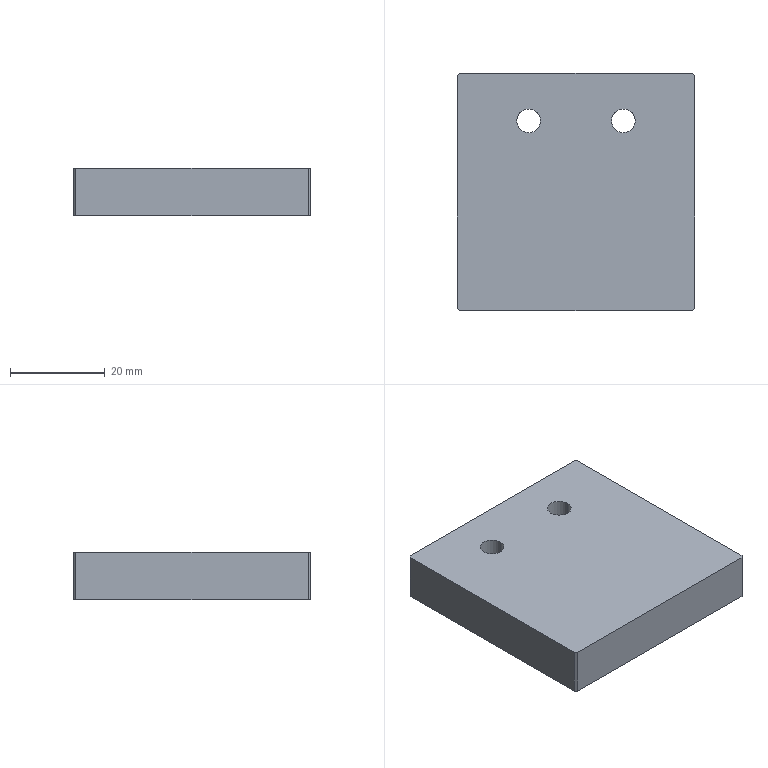Part | STEP file | 2027 Cylinder pad block | 1 solid | 14 faces | box 50 x 50 x 10 mm | volume 24602 mm3 | plane 10 | cylinder 4 | commonest cylinder face diameters 5 x4
STEP:
#1=CARTESIAN_POINT('',(0.,0.,0.));
#2=DIRECTION('',(0.,0.,1.));
#3=DIRECTION('',(1.,0.,0.));
#4=AXIS2_PLACEMENT_3D('',#1,#2,#3);
#5=CARTESIAN_POINT('',(-7.5,15.,0.));
#6=VERTEX_POINT('',#5);
#7=CARTESIAN_POINT('',(-7.5,15.,10.));
#8=VERTEX_POINT('',#7);
#9=CARTESIAN_POINT('',(-7.5,15.,10.));
#10=DIRECTION('',(0.,0.,1.));
#11=VECTOR('',#10,1.);
#12=LINE('',#9,#11);
#13=CARTESIAN_POINT('',(-10.,15.,10.));
#14=DIRECTION('',(0.,0.,1.));
#15=DIRECTION('',(1.,0.,0.));
#16=AXIS2_PLACEMENT_3D('',#13,#14,#15);
#17=CYLINDRICAL_SURFACE('',#16,2.5);
#18=CARTESIAN_POINT('',(6.283,0.));
#19=DIRECTION('',(0.,1.));
#20=VECTOR('',#19,1.);
#21=LINE('',#18,#20);
#22=(GEOMETRIC_REPRESENTATION_CONTEXT(2)PARAMETRIC_REPRESENTATION_CONTEXT()REPRESENTATION_CONTEXT('',''));
#23=DEFINITIONAL_REPRESENTATION('',(#21),#22);
#24=PCURVE('',#17,#23);
#25=CARTESIAN_POINT('',(-10.,15.,10.));
#26=DIRECTION('',(0.,0.,1.));
#27=DIRECTION('',(1.,0.,0.));
#28=AXIS2_PLACEMENT_3D('',#25,#26,#27);
#29=CYLINDRICAL_SURFACE('',#28,2.5);
#30=CARTESIAN_POINT('',(0.,0.));
#31=DIRECTION('',(0.,1.));
#32=VECTOR('',#31,1.);
#33=LINE('',#30,#32);
#34=(GEOMETRIC_REPRESENTATION_CONTEXT(2)PARAMETRIC_REPRESENTATION_CONTEXT()REPRESENTATION_CONTEXT('',''));
#35=DEFINITIONAL_REPRESENTATION('',(#33),#34);
#36=PCURVE('',#29,#35);
#37=SURFACE_CURVE('',#12,(#24,#36),.PCURVE_S1.);
#38=EDGE_CURVE('',#6,#8,#37,.T.);
#39=ORIENTED_EDGE('',*,*,#38,.T.);
#40=CARTESIAN_POINT('',(-12.5,15.,10.));
#41=VERTEX_POINT('',#40);
#42=CARTESIAN_POINT('',(-10.,15.,10.));
#43=DIRECTION('',(0.,0.,1.));
#44=DIRECTION('',(1.,0.,0.));
#45=AXIS2_PLACEMENT_3D('',#42,#43,#44);
#46=CIRCLE('',#45,2.5);
#47=CARTESIAN_POINT('',(0.,0.));
#48=DIRECTION('',(1.,0.));
#49=VECTOR('',#48,1.);
#50=LINE('',#47,#49);
#51=(GEOMETRIC_REPRESENTATION_CONTEXT(2)PARAMETRIC_REPRESENTATION_CONTEXT()REPRESENTATION_CONTEXT('',''));
#52=DEFINITIONAL_REPRESENTATION('',(#50),#51);
#53=PCURVE('',#17,#52);
#54=CARTESIAN_POINT('',(0.,0.,10.));
#55=DIRECTION('',(0.,0.,-1.));
#56=DIRECTION('',(-1.,0.,0.));
#57=AXIS2_PLACEMENT_3D('',#54,#55,#56);
#58=PLANE('',#57);
#59=CARTESIAN_POINT('',(7.5,15.));
#60=CARTESIAN_POINT('',(7.5,19.33));
#61=CARTESIAN_POINT('',(11.25,17.165));
#62=CARTESIAN_POINT('',(15.,15.));
#63=CARTESIAN_POINT('',(11.25,12.835));
#64=CARTESIAN_POINT('',(7.5,10.67));
#65=CARTESIAN_POINT('',(7.5,15.));
#66=(BOUNDED_CURVE()B_SPLINE_CURVE(2,(#59,#60,#61,#62,#63,#64,#65),.UNSPECIFIED.,.T.,.F.)B_SPLINE_CURVE_WITH_KNOTS((1,2,2,2,2,1),(-2.094,0.,2.094,4.189,6.283,8.378),.UNSPECIFIED.)CURVE()GEOMETRIC_REPRESENTATION_ITEM()RATIONAL_B_SPLINE_CURVE((1.,0.5,1.,0.5,1.,0.5,1.))REPRESENTATION_ITEM(''));
#67=(GEOMETRIC_REPRESENTATION_CONTEXT(2)PARAMETRIC_REPRESENTATION_CONTEXT()REPRESENTATION_CONTEXT('',''));
#68=DEFINITIONAL_REPRESENTATION('',(#66),#67);
#69=PCURVE('',#58,#68);
#70=SURFACE_CURVE('',#46,(#53,#69),.PCURVE_S1.);
#71=EDGE_CURVE('',#41,#8,#70,.T.);
#72=ORIENTED_EDGE('',*,*,#71,.F.);
#73=CARTESIAN_POINT('',(-12.5,15.,0.));
#74=VERTEX_POINT('',#73);
#75=CARTESIAN_POINT('',(-12.5,15.,10.));
#76=DIRECTION('',(0.,0.,1.));
#77=VECTOR('',#76,1.);
#78=LINE('',#75,#77);
#79=CARTESIAN_POINT('',(3.142,0.));
#80=DIRECTION('',(0.,1.));
#81=VECTOR('',#80,1.);
#82=LINE('',#79,#81);
#83=(GEOMETRIC_REPRESENTATION_CONTEXT(2)PARAMETRIC_REPRESENTATION_CONTEXT()REPRESENTATION_CONTEXT('',''));
#84=DEFINITIONAL_REPRESENTATION('',(#82),#83);
#85=PCURVE('',#17,#84);
#86=CARTESIAN_POINT('',(3.142,0.));
#87=DIRECTION('',(0.,1.));
#88=VECTOR('',#87,1.);
#89=LINE('',#86,#88);
#90=(GEOMETRIC_REPRESENTATION_CONTEXT(2)PARAMETRIC_REPRESENTATION_CONTEXT()REPRESENTATION_CONTEXT('',''));
#91=DEFINITIONAL_REPRESENTATION('',(#89),#90);
#92=PCURVE('',#29,#91);
#93=SURFACE_CURVE('',#78,(#85,#92),.PCURVE_S1.);
#94=EDGE_CURVE('',#74,#41,#93,.T.);
#95=ORIENTED_EDGE('',*,*,#94,.F.);
#96=CARTESIAN_POINT('',(-10.,15.,0.));
#97=DIRECTION('',(0.,0.,1.));
#98=DIRECTION('',(1.,0.,0.));
#99=AXIS2_PLACEMENT_3D('',#96,#97,#98);
#100=CIRCLE('',#99,2.5);
#101=CARTESIAN_POINT('',(0.,-10.));
#102=DIRECTION('',(1.,0.));
#103=VECTOR('',#102,1.);
#104=LINE('',#101,#103);
#105=(GEOMETRIC_REPRESENTATION_CONTEXT(2)PARAMETRIC_REPRESENTATION_CONTEXT()REPRESENTATION_CONTEXT('',''));
#106=DEFINITIONAL_REPRESENTATION('',(#104),#105);
#107=PCURVE('',#17,#106);
#108=CARTESIAN_POINT('',(0.,0.,0.));
#109=DIRECTION('',(0.,0.,-1.));
#110=DIRECTION('',(-1.,0.,0.));
#111=AXIS2_PLACEMENT_3D('',#108,#109,#110);
#112=PLANE('',#111);
#113=CARTESIAN_POINT('',(7.5,15.));
#114=CARTESIAN_POINT('',(7.5,19.33));
#115=CARTESIAN_POINT('',(11.25,17.165));
#116=CARTESIAN_POINT('',(15.,15.));
#117=CARTESIAN_POINT('',(11.25,12.835));
#118=CARTESIAN_POINT('',(7.5,10.67));
#119=CARTESIAN_POINT('',(7.5,15.));
#120=(BOUNDED_CURVE()B_SPLINE_CURVE(2,(#113,#114,#115,#116,#117,#118,#119),.UNSPECIFIED.,.T.,.F.)B_SPLINE_CURVE_WITH_KNOTS((1,2,2,2,2,1),(-2.094,0.,2.094,4.189,6.283,8.378),.UNSPECIFIED.)CURVE()GEOMETRIC_REPRESENTATION_ITEM()RATIONAL_B_SPLINE_CURVE((1.,0.5,1.,0.5,1.,0.5,1.))REPRESENTATION_ITEM(''));
#121=(GEOMETRIC_REPRESENTATION_CONTEXT(2)PARAMETRIC_REPRESENTATION_CONTEXT()REPRESENTATION_CONTEXT('',''));
#122=DEFINITIONAL_REPRESENTATION('',(#120),#121);
#123=PCURVE('',#112,#122);
#124=SURFACE_CURVE('',#100,(#107,#123),.PCURVE_S1.);
#125=EDGE_CURVE('',#74,#6,#124,.T.);
#126=ORIENTED_EDGE('',*,*,#125,.T.);
#127=EDGE_LOOP('',(#39,#72,#95,#126));
#128=FACE_BOUND('',#127,.F.);
#129=ADVANCED_FACE('',(#128),#17,.F.);
#130=CARTESIAN_POINT('',(12.5,15.,0.));
#131=VERTEX_POINT('',#130);
#132=CARTESIAN_POINT('',(12.5,15.,10.));
#133=VERTEX_POINT('',#132);
#134=CARTESIAN_POINT('',(12.5,15.,10.));
#135=DIRECTION('',(0.,0.,1.));
#136=VECTOR('',#135,1.);
#137=LINE('',#134,#136);
#138=CARTESIAN_POINT('',(10.,15.,10.));
#139=DIRECTION('',(0.,0.,1.));
#140=DIRECTION('',(1.,0.,0.));
#141=AXIS2_PLACEMENT_3D('',#138,#139,#140);
#142=CYLINDRICAL_SURFACE('',#141,2.5);
#143=CARTESIAN_POINT('',(6.283,0.));
#144=DIRECTION('',(0.,1.));
#145=VECTOR('',#144,1.);
#146=LINE('',#143,#145);
#147=(GEOMETRIC_REPRESENTATION_CONTEXT(2)PARAMETRIC_REPRESENTATION_CONTEXT()REPRESENTATION_CONTEXT('',''));
#148=DEFINITIONAL_REPRESENTATION('',(#146),#147);
#149=PCURVE('',#142,#148);
#150=CARTESIAN_POINT('',(10.,15.,10.));
#151=DIRECTION('',(0.,0.,1.));
#152=DIRECTION('',(1.,0.,0.));
#153=AXIS2_PLACEMENT_3D('',#150,#151,#152);
#154=CYLINDRICAL_SURFACE('',#153,2.5);
#155=CARTESIAN_POINT('',(0.,0.));
#156=DIRECTION('',(0.,1.));
#157=VECTOR('',#156,1.);
#158=LINE('',#155,#157);
#159=(GEOMETRIC_REPRESENTATION_CONTEXT(2)PARAMETRIC_REPRESENTATION_CONTEXT()REPRESENTATION_CONTEXT('',''));
#160=DEFINITIONAL_REPRESENTATION('',(#158),#159);
#161=PCURVE('',#154,#160);
#162=SURFACE_CURVE('',#137,(#149,#161),.PCURVE_S1.);
#163=EDGE_CURVE('',#131,#133,#162,.T.);
#164=ORIENTED_EDGE('',*,*,#163,.T.);
#165=CARTESIAN_POINT('',(7.5,15.,10.));
#166=VERTEX_POINT('',#165);
#167=CARTESIAN_POINT('',(10.,15.,10.));
#168=DIRECTION('',(0.,0.,1.));
#169=DIRECTION('',(1.,0.,0.));
#170=AXIS2_PLACEMENT_3D('',#167,#168,#169);
#171=CIRCLE('',#170,2.5);
#172=CARTESIAN_POINT('',(0.,0.));
#173=DIRECTION('',(1.,0.));
#174=VECTOR('',#173,1.);
#175=LINE('',#172,#174);
#176=(GEOMETRIC_REPRESENTATION_CONTEXT(2)PARAMETRIC_REPRESENTATION_CONTEXT()REPRESENTATION_CONTEXT('',''));
#177=DEFINITIONAL_REPRESENTATION('',(#175),#176);
#178=PCURVE('',#142,#177);
#179=CARTESIAN_POINT('',(-12.5,15.));
#180=CARTESIAN_POINT('',(-12.5,19.33));
#181=CARTESIAN_POINT('',(-8.75,17.165));
#182=CARTESIAN_POINT('',(-5.,15.));
#183=CARTESIAN_POINT('',(-8.75,12.835));
#184=CARTESIAN_POINT('',(-12.5,10.67));
#185=CARTESIAN_POINT('',(-12.5,15.));
#186=(BOUNDED_CURVE()B_SPLINE_CURVE(2,(#179,#180,#181,#182,#183,#184,#185),.UNSPECIFIED.,.T.,.F.)B_SPLINE_CURVE_WITH_KNOTS((1,2,2,2,2,1),(-2.094,0.,2.094,4.189,6.283,8.378),.UNSPECIFIED.)CURVE()GEOMETRIC_REPRESENTATION_ITEM()RATIONAL_B_SPLINE_CURVE((1.,0.5,1.,0.5,1.,0.5,1.))REPRESENTATION_ITEM(''));
#187=(GEOMETRIC_REPRESENTATION_CONTEXT(2)PARAMETRIC_REPRESENTATION_CONTEXT()REPRESENTATION_CONTEXT('',''));
#188=DEFINITIONAL_REPRESENTATION('',(#186),#187);
#189=PCURVE('',#58,#188);
#190=SURFACE_CURVE('',#171,(#178,#189),.PCURVE_S1.);
#191=EDGE_CURVE('',#166,#133,#190,.T.);
#192=ORIENTED_EDGE('',*,*,#191,.F.);
#193=CARTESIAN_POINT('',(7.5,15.,0.));
#194=VERTEX_POINT('',#193);
#195=CARTESIAN_POINT('',(7.5,15.,10.));
#196=DIRECTION('',(0.,0.,1.));
#197=VECTOR('',#196,1.);
#198=LINE('',#195,#197);
#199=CARTESIAN_POINT('',(3.142,0.));
#200=DIRECTION('',(0.,1.));
#201=VECTOR('',#200,1.);
#202=LINE('',#199,#201);
#203=(GEOMETRIC_REPRESENTATION_CONTEXT(2)PARAMETRIC_REPRESENTATION_CONTEXT()REPRESENTATION_CONTEXT('',''));
#204=DEFINITIONAL_REPRESENTATION('',(#202),#203);
#205=PCURVE('',#142,#204);
#206=CARTESIAN_POINT('',(3.142,0.));
#207=DIRECTION('',(0.,1.));
#208=VECTOR('',#207,1.);
#209=LINE('',#206,#208);
#210=(GEOMETRIC_REPRESENTATION_CONTEXT(2)PARAMETRIC_REPRESENTATION_CONTEXT()REPRESENTATION_CONTEXT('',''));
#211=DEFINITIONAL_REPRESENTATION('',(#209),#210);
#212=PCURVE('',#154,#211);
#213=SURFACE_CURVE('',#198,(#205,#212),.PCURVE_S1.);
#214=EDGE_CURVE('',#194,#166,#213,.T.);
#215=ORIENTED_EDGE('',*,*,#214,.F.);
#216=CARTESIAN_POINT('',(10.,15.,0.));
#217=DIRECTION('',(0.,0.,1.));
#218=DIRECTION('',(1.,0.,0.));
#219=AXIS2_PLACEMENT_3D('',#216,#217,#218);
#220=CIRCLE('',#219,2.5);
#221=CARTESIAN_POINT('',(0.,-10.));
#222=DIRECTION('',(1.,0.));
#223=VECTOR('',#222,1.);
#224=LINE('',#221,#223);
#225=(GEOMETRIC_REPRESENTATION_CONTEXT(2)PARAMETRIC_REPRESENTATION_CONTEXT()REPRESENTATION_CONTEXT('',''));
#226=DEFINITIONAL_REPRESENTATION('',(#224),#225);
#227=PCURVE('',#142,#226);
#228=CARTESIAN_POINT('',(-12.5,15.));
#229=CARTESIAN_POINT('',(-12.5,19.33));
#230=CARTESIAN_POINT('',(-8.75,17.165));
#231=CARTESIAN_POINT('',(-5.,15.));
#232=CARTESIAN_POINT('',(-8.75,12.835));
#233=CARTESIAN_POINT('',(-12.5,10.67));
#234=CARTESIAN_POINT('',(-12.5,15.));
#235=(BOUNDED_CURVE()B_SPLINE_CURVE(2,(#228,#229,#230,#231,#232,#233,#234),.UNSPECIFIED.,.T.,.F.)B_SPLINE_CURVE_WITH_KNOTS((1,2,2,2,2,1),(-2.094,0.,2.094,4.189,6.283,8.378),.UNSPECIFIED.)CURVE()GEOMETRIC_REPRESENTATION_ITEM()RATIONAL_B_SPLINE_CURVE((1.,0.5,1.,0.5,1.,0.5,1.))REPRESENTATION_ITEM(''));
#236=(GEOMETRIC_REPRESENTATION_CONTEXT(2)PARAMETRIC_REPRESENTATION_CONTEXT()REPRESENTATION_CONTEXT('',''));
#237=DEFINITIONAL_REPRESENTATION('',(#235),#236);
#238=PCURVE('',#112,#237);
#239=SURFACE_CURVE('',#220,(#227,#238),.PCURVE_S1.);
#240=EDGE_CURVE('',#194,#131,#239,.T.);
#241=ORIENTED_EDGE('',*,*,#240,.T.);
#242=EDGE_LOOP('',(#164,#192,#215,#241));
#243=FACE_BOUND('',#242,.F.);
#244=ADVANCED_FACE('',(#243),#142,.F.);
#245=CARTESIAN_POINT('',(25.,-24.5,0.));
#246=VERTEX_POINT('',#245);
#247=CARTESIAN_POINT('',(25.,24.5,0.));
#248=VERTEX_POINT('',#247);
#249=CARTESIAN_POINT('',(25.,-25.,0.));
#250=DIRECTION('',(0.,1.,0.));
#251=VECTOR('',#250,1.);
#252=LINE('',#249,#251);
#253=CARTESIAN_POINT('',(25.,-25.,10.));
#254=DIRECTION('',(-1.,0.,0.));
#255=DIRECTION('',(0.,0.,1.));
#256=AXIS2_PLACEMENT_3D('',#253,#254,#255);
#257=PLANE('',#256);
#258=CARTESIAN_POINT('',(-10.,0.));
#259=DIRECTION('',(0.,1.));
#260=VECTOR('',#259,1.);
#261=LINE('',#258,#260);
#262=(GEOMETRIC_REPRESENTATION_CONTEXT(2)PARAMETRIC_REPRESENTATION_CONTEXT()REPRESENTATION_CONTEXT('',''));
#263=DEFINITIONAL_REPRESENTATION('',(#261),#262);
#264=PCURVE('',#257,#263);
#265=CARTESIAN_POINT('',(-25.,-25.));
#266=DIRECTION('',(0.,1.));
#267=VECTOR('',#266,1.);
#268=LINE('',#265,#267);
#269=(GEOMETRIC_REPRESENTATION_CONTEXT(2)PARAMETRIC_REPRESENTATION_CONTEXT()REPRESENTATION_CONTEXT('',''));
#270=DEFINITIONAL_REPRESENTATION('',(#268),#269);
#271=PCURVE('',#112,#270);
#272=SURFACE_CURVE('',#252,(#264,#271),.PCURVE_S1.);
#273=EDGE_CURVE('',#246,#248,#272,.T.);
#274=ORIENTED_EDGE('',*,*,#273,.T.);
#275=CARTESIAN_POINT('',(25.,24.5,10.));
#276=VERTEX_POINT('',#275);
#277=CARTESIAN_POINT('',(25.,24.5,10.));
#278=DIRECTION('',(0.,0.,1.));
#279=VECTOR('',#278,1.);
#280=LINE('',#277,#279);
#281=CARTESIAN_POINT('',(0.,49.5));
#282=DIRECTION('',(1.,0.));
#283=VECTOR('',#282,1.);
#284=LINE('',#281,#283);
#285=(GEOMETRIC_REPRESENTATION_CONTEXT(2)PARAMETRIC_REPRESENTATION_CONTEXT()REPRESENTATION_CONTEXT('',''));
#286=DEFINITIONAL_REPRESENTATION('',(#284),#285);
#287=PCURVE('',#257,#286);
#288=CARTESIAN_POINT('',(24.5,25.,10.));
#289=DIRECTION('',(-0.7071,-0.7071,0.));
#290=DIRECTION('',(0.,0.,-1.));
#291=AXIS2_PLACEMENT_3D('',#288,#289,#290);
#292=PLANE('',#291);
#293=CARTESIAN_POINT('',(0.,0.7071));
#294=DIRECTION('',(-1.,0.));
#295=VECTOR('',#294,1.);
#296=LINE('',#293,#295);
#297=(GEOMETRIC_REPRESENTATION_CONTEXT(2)PARAMETRIC_REPRESENTATION_CONTEXT()REPRESENTATION_CONTEXT('',''));
#298=DEFINITIONAL_REPRESENTATION('',(#296),#297);
#299=PCURVE('',#292,#298);
#300=SURFACE_CURVE('',#280,(#287,#299),.PCURVE_S1.);
#301=EDGE_CURVE('',#248,#276,#300,.T.);
#302=ORIENTED_EDGE('',*,*,#301,.T.);
#303=CARTESIAN_POINT('',(25.,-24.5,10.));
#304=VERTEX_POINT('',#303);
#305=CARTESIAN_POINT('',(25.,-25.,10.));
#306=DIRECTION('',(0.,1.,0.));
#307=VECTOR('',#306,1.);
#308=LINE('',#305,#307);
#309=CARTESIAN_POINT('',(0.,0.));
#310=DIRECTION('',(0.,1.));
#311=VECTOR('',#310,1.);
#312=LINE('',#309,#311);
#313=(GEOMETRIC_REPRESENTATION_CONTEXT(2)PARAMETRIC_REPRESENTATION_CONTEXT()REPRESENTATION_CONTEXT('',''));
#314=DEFINITIONAL_REPRESENTATION('',(#312),#313);
#315=PCURVE('',#257,#314);
#316=CARTESIAN_POINT('',(-25.,-25.));
#317=DIRECTION('',(0.,1.));
#318=VECTOR('',#317,1.);
#319=LINE('',#316,#318);
#320=(GEOMETRIC_REPRESENTATION_CONTEXT(2)PARAMETRIC_REPRESENTATION_CONTEXT()REPRESENTATION_CONTEXT('',''));
#321=DEFINITIONAL_REPRESENTATION('',(#319),#320);
#322=PCURVE('',#58,#321);
#323=SURFACE_CURVE('',#308,(#315,#322),.PCURVE_S1.);
#324=EDGE_CURVE('',#304,#276,#323,.T.);
#325=ORIENTED_EDGE('',*,*,#324,.F.);
#326=CARTESIAN_POINT('',(25.,-24.5,10.));
#327=DIRECTION('',(0.,0.,-1.));
#328=VECTOR('',#327,1.);
#329=LINE('',#326,#328);
#330=CARTESIAN_POINT('',(0.,0.5));
#331=DIRECTION('',(-1.,0.));
#332=VECTOR('',#331,1.);
#333=LINE('',#330,#332);
#334=(GEOMETRIC_REPRESENTATION_CONTEXT(2)PARAMETRIC_REPRESENTATION_CONTEXT()REPRESENTATION_CONTEXT('',''));
#335=DEFINITIONAL_REPRESENTATION('',(#333),#334);
#336=PCURVE('',#257,#335);
#337=CARTESIAN_POINT('',(25.,-24.5,10.));
#338=DIRECTION('',(-0.7071,0.7071,0.));
#339=DIRECTION('',(0.,0.,-1.));
#340=AXIS2_PLACEMENT_3D('',#337,#338,#339);
#341=PLANE('',#340);
#342=CARTESIAN_POINT('',(0.,0.));
#343=DIRECTION('',(1.,0.));
#344=VECTOR('',#343,1.);
#345=LINE('',#342,#344);
#346=(GEOMETRIC_REPRESENTATION_CONTEXT(2)PARAMETRIC_REPRESENTATION_CONTEXT()REPRESENTATION_CONTEXT('',''));
#347=DEFINITIONAL_REPRESENTATION('',(#345),#346);
#348=PCURVE('',#341,#347);
#349=SURFACE_CURVE('',#329,(#336,#348),.PCURVE_S1.);
#350=EDGE_CURVE('',#304,#246,#349,.T.);
#351=ORIENTED_EDGE('',*,*,#350,.T.);
#352=EDGE_LOOP('',(#274,#302,#325,#351));
#353=FACE_BOUND('',#352,.T.);
#354=ADVANCED_FACE('',(#353),#257,.F.);
#355=CARTESIAN_POINT('',(24.5,25.,10.));
#356=VERTEX_POINT('',#355);
#357=CARTESIAN_POINT('',(-24.5,25.,10.));
#358=VERTEX_POINT('',#357);
#359=CARTESIAN_POINT('',(-25.,25.,10.));
#360=DIRECTION('',(-1.,0.,0.));
#361=VECTOR('',#360,1.);
#362=LINE('',#359,#361);
#363=CARTESIAN_POINT('',(-25.,25.,10.));
#364=DIRECTION('',(0.,-1.,0.));
#365=DIRECTION('',(0.,0.,-1.));
#366=AXIS2_PLACEMENT_3D('',#363,#364,#365);
#367=PLANE('',#366);
#368=CARTESIAN_POINT('',(0.,0.));
#369=DIRECTION('',(0.,-1.));
#370=VECTOR('',#369,1.);
#371=LINE('',#368,#370);
#372=(GEOMETRIC_REPRESENTATION_CONTEXT(2)PARAMETRIC_REPRESENTATION_CONTEXT()REPRESENTATION_CONTEXT('',''));
#373=DEFINITIONAL_REPRESENTATION('',(#371),#372);
#374=PCURVE('',#367,#373);
#375=CARTESIAN_POINT('',(25.,25.));
#376=DIRECTION('',(1.,0.));
#377=VECTOR('',#376,1.);
#378=LINE('',#375,#377);
#379=(GEOMETRIC_REPRESENTATION_CONTEXT(2)PARAMETRIC_REPRESENTATION_CONTEXT()REPRESENTATION_CONTEXT('',''));
#380=DEFINITIONAL_REPRESENTATION('',(#378),#379);
#381=PCURVE('',#58,#380);
#382=SURFACE_CURVE('',#362,(#374,#381),.PCURVE_S1.);
#383=EDGE_CURVE('',#356,#358,#382,.T.);
#384=ORIENTED_EDGE('',*,*,#383,.F.);
#385=CARTESIAN_POINT('',(24.5,25.,0.));
#386=VERTEX_POINT('',#385);
#387=CARTESIAN_POINT('',(24.5,25.,10.));
#388=DIRECTION('',(0.,0.,-1.));
#389=VECTOR('',#388,1.);
#390=LINE('',#387,#389);
#391=CARTESIAN_POINT('',(0.,49.5));
#392=DIRECTION('',(1.,0.));
#393=VECTOR('',#392,1.);
#394=LINE('',#391,#393);
#395=(GEOMETRIC_REPRESENTATION_CONTEXT(2)PARAMETRIC_REPRESENTATION_CONTEXT()REPRESENTATION_CONTEXT('',''));
#396=DEFINITIONAL_REPRESENTATION('',(#394),#395);
#397=PCURVE('',#367,#396);
#398=CARTESIAN_POINT('',(0.,0.));
#399=DIRECTION('',(1.,0.));
#400=VECTOR('',#399,1.);
#401=LINE('',#398,#400);
#402=(GEOMETRIC_REPRESENTATION_CONTEXT(2)PARAMETRIC_REPRESENTATION_CONTEXT()REPRESENTATION_CONTEXT('',''));
#403=DEFINITIONAL_REPRESENTATION('',(#401),#402);
#404=PCURVE('',#292,#403);
#405=SURFACE_CURVE('',#390,(#397,#404),.PCURVE_S1.);
#406=EDGE_CURVE('',#356,#386,#405,.T.);
#407=ORIENTED_EDGE('',*,*,#406,.T.);
#408=CARTESIAN_POINT('',(-24.5,25.,0.));
#409=VERTEX_POINT('',#408);
#410=CARTESIAN_POINT('',(-25.,25.,0.));
#411=DIRECTION('',(-1.,0.,0.));
#412=VECTOR('',#411,1.);
#413=LINE('',#410,#412);
#414=CARTESIAN_POINT('',(10.,0.));
#415=DIRECTION('',(0.,-1.));
#416=VECTOR('',#415,1.);
#417=LINE('',#414,#416);
#418=(GEOMETRIC_REPRESENTATION_CONTEXT(2)PARAMETRIC_REPRESENTATION_CONTEXT()REPRESENTATION_CONTEXT('',''));
#419=DEFINITIONAL_REPRESENTATION('',(#417),#418);
#420=PCURVE('',#367,#419);
#421=CARTESIAN_POINT('',(25.,25.));
#422=DIRECTION('',(1.,0.));
#423=VECTOR('',#422,1.);
#424=LINE('',#421,#423);
#425=(GEOMETRIC_REPRESENTATION_CONTEXT(2)PARAMETRIC_REPRESENTATION_CONTEXT()REPRESENTATION_CONTEXT('',''));
#426=DEFINITIONAL_REPRESENTATION('',(#424),#425);
#427=PCURVE('',#112,#426);
#428=SURFACE_CURVE('',#413,(#420,#427),.PCURVE_S1.);
#429=EDGE_CURVE('',#386,#409,#428,.T.);
#430=ORIENTED_EDGE('',*,*,#429,.T.);
#431=CARTESIAN_POINT('',(-24.5,25.,10.));
#432=DIRECTION('',(0.,0.,1.));
#433=VECTOR('',#432,1.);
#434=LINE('',#431,#433);
#435=CARTESIAN_POINT('',(0.,0.5));
#436=DIRECTION('',(-1.,0.));
#437=VECTOR('',#436,1.);
#438=LINE('',#435,#437);
#439=(GEOMETRIC_REPRESENTATION_CONTEXT(2)PARAMETRIC_REPRESENTATION_CONTEXT()REPRESENTATION_CONTEXT('',''));
#440=DEFINITIONAL_REPRESENTATION('',(#438),#439);
#441=PCURVE('',#367,#440);
#442=CARTESIAN_POINT('',(-25.,24.5,10.));
#443=DIRECTION('',(0.7071,-0.7071,0.));
#444=DIRECTION('',(0.,0.,-1.));
#445=AXIS2_PLACEMENT_3D('',#442,#443,#444);
#446=PLANE('',#445);
#447=CARTESIAN_POINT('',(0.,0.7071));
#448=DIRECTION('',(-1.,0.));
#449=VECTOR('',#448,1.);
#450=LINE('',#447,#449);
#451=(GEOMETRIC_REPRESENTATION_CONTEXT(2)PARAMETRIC_REPRESENTATION_CONTEXT()REPRESENTATION_CONTEXT('',''));
#452=DEFINITIONAL_REPRESENTATION('',(#450),#451);
#453=PCURVE('',#446,#452);
#454=SURFACE_CURVE('',#434,(#441,#453),.PCURVE_S1.);
#455=EDGE_CURVE('',#409,#358,#454,.T.);
#456=ORIENTED_EDGE('',*,*,#455,.T.);
#457=EDGE_LOOP('',(#384,#407,#430,#456));
#458=FACE_BOUND('',#457,.T.);
#459=ADVANCED_FACE('',(#458),#367,.F.);
#460=CARTESIAN_POINT('',(-25.,24.5,0.));
#461=VERTEX_POINT('',#460);
#462=CARTESIAN_POINT('',(-25.,-24.5,0.));
#463=VERTEX_POINT('',#462);
#464=CARTESIAN_POINT('',(-25.,-25.,0.));
#465=DIRECTION('',(0.,-1.,0.));
#466=VECTOR('',#465,1.);
#467=LINE('',#464,#466);
#468=CARTESIAN_POINT('',(-25.,-25.,10.));
#469=DIRECTION('',(1.,0.,0.));
#470=DIRECTION('',(0.,0.,-1.));
#471=AXIS2_PLACEMENT_3D('',#468,#469,#470);
#472=PLANE('',#471);
#473=CARTESIAN_POINT('',(10.,0.));
#474=DIRECTION('',(0.,-1.));
#475=VECTOR('',#474,1.);
#476=LINE('',#473,#475);
#477=(GEOMETRIC_REPRESENTATION_CONTEXT(2)PARAMETRIC_REPRESENTATION_CONTEXT()REPRESENTATION_CONTEXT('',''));
#478=DEFINITIONAL_REPRESENTATION('',(#476),#477);
#479=PCURVE('',#472,#478);
#480=CARTESIAN_POINT('',(25.,-25.));
#481=DIRECTION('',(0.,-1.));
#482=VECTOR('',#481,1.);
#483=LINE('',#480,#482);
#484=(GEOMETRIC_REPRESENTATION_CONTEXT(2)PARAMETRIC_REPRESENTATION_CONTEXT()REPRESENTATION_CONTEXT('',''));
#485=DEFINITIONAL_REPRESENTATION('',(#483),#484);
#486=PCURVE('',#112,#485);
#487=SURFACE_CURVE('',#467,(#479,#486),.PCURVE_S1.);
#488=EDGE_CURVE('',#461,#463,#487,.T.);
#489=ORIENTED_EDGE('',*,*,#488,.T.);
#490=CARTESIAN_POINT('',(-25.,-24.5,10.));
#491=VERTEX_POINT('',#490);
#492=CARTESIAN_POINT('',(-25.,-24.5,10.));
#493=DIRECTION('',(0.,0.,1.));
#494=VECTOR('',#493,1.);
#495=LINE('',#492,#494);
#496=CARTESIAN_POINT('',(0.,0.5));
#497=DIRECTION('',(-1.,0.));
#498=VECTOR('',#497,1.);
#499=LINE('',#496,#498);
#500=(GEOMETRIC_REPRESENTATION_CONTEXT(2)PARAMETRIC_REPRESENTATION_CONTEXT()REPRESENTATION_CONTEXT('',''));
#501=DEFINITIONAL_REPRESENTATION('',(#499),#500);
#502=PCURVE('',#472,#501);
#503=CARTESIAN_POINT('',(-24.5,-25.,10.));
#504=DIRECTION('',(0.7071,0.7071,0.));
#505=DIRECTION('',(0.,0.,-1.));
#506=AXIS2_PLACEMENT_3D('',#503,#504,#505);
#507=PLANE('',#506);
#508=CARTESIAN_POINT('',(0.,0.7071));
#509=DIRECTION('',(-1.,0.));
#510=VECTOR('',#509,1.);
#511=LINE('',#508,#510);
#512=(GEOMETRIC_REPRESENTATION_CONTEXT(2)PARAMETRIC_REPRESENTATION_CONTEXT()REPRESENTATION_CONTEXT('',''));
#513=DEFINITIONAL_REPRESENTATION('',(#511),#512);
#514=PCURVE('',#507,#513);
#515=SURFACE_CURVE('',#495,(#502,#514),.PCURVE_S1.);
#516=EDGE_CURVE('',#463,#491,#515,.T.);
#517=ORIENTED_EDGE('',*,*,#516,.T.);
#518=CARTESIAN_POINT('',(-25.,24.5,10.));
#519=VERTEX_POINT('',#518);
#520=CARTESIAN_POINT('',(-25.,-25.,10.));
#521=DIRECTION('',(0.,-1.,0.));
#522=VECTOR('',#521,1.);
#523=LINE('',#520,#522);
#524=CARTESIAN_POINT('',(0.,0.));
#525=DIRECTION('',(0.,-1.));
#526=VECTOR('',#525,1.);
#527=LINE('',#524,#526);
#528=(GEOMETRIC_REPRESENTATION_CONTEXT(2)PARAMETRIC_REPRESENTATION_CONTEXT()REPRESENTATION_CONTEXT('',''));
#529=DEFINITIONAL_REPRESENTATION('',(#527),#528);
#530=PCURVE('',#472,#529);
#531=CARTESIAN_POINT('',(25.,-25.));
#532=DIRECTION('',(0.,-1.));
#533=VECTOR('',#532,1.);
#534=LINE('',#531,#533);
#535=(GEOMETRIC_REPRESENTATION_CONTEXT(2)PARAMETRIC_REPRESENTATION_CONTEXT()REPRESENTATION_CONTEXT('',''));
#536=DEFINITIONAL_REPRESENTATION('',(#534),#535);
#537=PCURVE('',#58,#536);
#538=SURFACE_CURVE('',#523,(#530,#537),.PCURVE_S1.);
#539=EDGE_CURVE('',#519,#491,#538,.T.);
#540=ORIENTED_EDGE('',*,*,#539,.F.);
#541=CARTESIAN_POINT('',(-25.,24.5,10.));
#542=DIRECTION('',(0.,0.,-1.));
#543=VECTOR('',#542,1.);
#544=LINE('',#541,#543);
#545=CARTESIAN_POINT('',(0.,49.5));
#546=DIRECTION('',(1.,0.));
#547=VECTOR('',#546,1.);
#548=LINE('',#545,#547);
#549=(GEOMETRIC_REPRESENTATION_CONTEXT(2)PARAMETRIC_REPRESENTATION_CONTEXT()REPRESENTATION_CONTEXT('',''));
#550=DEFINITIONAL_REPRESENTATION('',(#548),#549);
#551=PCURVE('',#472,#550);
#552=CARTESIAN_POINT('',(0.,0.));
#553=DIRECTION('',(1.,0.));
#554=VECTOR('',#553,1.);
#555=LINE('',#552,#554);
#556=(GEOMETRIC_REPRESENTATION_CONTEXT(2)PARAMETRIC_REPRESENTATION_CONTEXT()REPRESENTATION_CONTEXT('',''));
#557=DEFINITIONAL_REPRESENTATION('',(#555),#556);
#558=PCURVE('',#446,#557);
#559=SURFACE_CURVE('',#544,(#551,#558),.PCURVE_S1.);
#560=EDGE_CURVE('',#519,#461,#559,.T.);
#561=ORIENTED_EDGE('',*,*,#560,.T.);
#562=EDGE_LOOP('',(#489,#517,#540,#561));
#563=FACE_BOUND('',#562,.T.);
#564=ADVANCED_FACE('',(#563),#472,.F.);
#565=CARTESIAN_POINT('',(-24.5,-25.,0.));
#566=VERTEX_POINT('',#565);
#567=CARTESIAN_POINT('',(24.5,-25.,0.));
#568=VERTEX_POINT('',#567);
#569=CARTESIAN_POINT('',(-25.,-25.,0.));
#570=DIRECTION('',(1.,0.,0.));
#571=VECTOR('',#570,1.);
#572=LINE('',#569,#571);
#573=CARTESIAN_POINT('',(-25.,-25.,10.));
#574=DIRECTION('',(0.,1.,0.));
#575=DIRECTION('',(0.,0.,1.));
#576=AXIS2_PLACEMENT_3D('',#573,#574,#575);
#577=PLANE('',#576);
#578=CARTESIAN_POINT('',(-10.,0.));
#579=DIRECTION('',(0.,1.));
#580=VECTOR('',#579,1.);
#581=LINE('',#578,#580);
#582=(GEOMETRIC_REPRESENTATION_CONTEXT(2)PARAMETRIC_REPRESENTATION_CONTEXT()REPRESENTATION_CONTEXT('',''));
#583=DEFINITIONAL_REPRESENTATION('',(#581),#582);
#584=PCURVE('',#577,#583);
#585=CARTESIAN_POINT('',(25.,-25.));
#586=DIRECTION('',(-1.,0.));
#587=VECTOR('',#586,1.);
#588=LINE('',#585,#587);
#589=(GEOMETRIC_REPRESENTATION_CONTEXT(2)PARAMETRIC_REPRESENTATION_CONTEXT()REPRESENTATION_CONTEXT('',''));
#590=DEFINITIONAL_REPRESENTATION('',(#588),#589);
#591=PCURVE('',#112,#590);
#592=SURFACE_CURVE('',#572,(#584,#591),.PCURVE_S1.);
#593=EDGE_CURVE('',#566,#568,#592,.T.);
#594=ORIENTED_EDGE('',*,*,#593,.T.);
#595=CARTESIAN_POINT('',(24.5,-25.,10.));
#596=VERTEX_POINT('',#595);
#597=CARTESIAN_POINT('',(24.5,-25.,10.));
#598=DIRECTION('',(0.,0.,1.));
#599=VECTOR('',#598,1.);
#600=LINE('',#597,#599);
#601=CARTESIAN_POINT('',(0.,49.5));
#602=DIRECTION('',(1.,0.));
#603=VECTOR('',#602,1.);
#604=LINE('',#601,#603);
#605=(GEOMETRIC_REPRESENTATION_CONTEXT(2)PARAMETRIC_REPRESENTATION_CONTEXT()REPRESENTATION_CONTEXT('',''));
#606=DEFINITIONAL_REPRESENTATION('',(#604),#605);
#607=PCURVE('',#577,#606);
#608=CARTESIAN_POINT('',(0.,0.7071));
#609=DIRECTION('',(-1.,0.));
#610=VECTOR('',#609,1.);
#611=LINE('',#608,#610);
#612=(GEOMETRIC_REPRESENTATION_CONTEXT(2)PARAMETRIC_REPRESENTATION_CONTEXT()REPRESENTATION_CONTEXT('',''));
#613=DEFINITIONAL_REPRESENTATION('',(#611),#612);
#614=PCURVE('',#341,#613);
#615=SURFACE_CURVE('',#600,(#607,#614),.PCURVE_S1.);
#616=EDGE_CURVE('',#568,#596,#615,.T.);
#617=ORIENTED_EDGE('',*,*,#616,.T.);
#618=CARTESIAN_POINT('',(-24.5,-25.,10.));
#619=VERTEX_POINT('',#618);
#620=CARTESIAN_POINT('',(-25.,-25.,10.));
#621=DIRECTION('',(1.,0.,0.));
#622=VECTOR('',#621,1.);
#623=LINE('',#620,#622);
#624=CARTESIAN_POINT('',(0.,0.));
#625=DIRECTION('',(0.,1.));
#626=VECTOR('',#625,1.);
#627=LINE('',#624,#626);
#628=(GEOMETRIC_REPRESENTATION_CONTEXT(2)PARAMETRIC_REPRESENTATION_CONTEXT()REPRESENTATION_CONTEXT('',''));
#629=DEFINITIONAL_REPRESENTATION('',(#627),#628);
#630=PCURVE('',#577,#629);
#631=CARTESIAN_POINT('',(25.,-25.));
#632=DIRECTION('',(-1.,0.));
#633=VECTOR('',#632,1.);
#634=LINE('',#631,#633);
#635=(GEOMETRIC_REPRESENTATION_CONTEXT(2)PARAMETRIC_REPRESENTATION_CONTEXT()REPRESENTATION_CONTEXT('',''));
#636=DEFINITIONAL_REPRESENTATION('',(#634),#635);
#637=PCURVE('',#58,#636);
#638=SURFACE_CURVE('',#623,(#630,#637),.PCURVE_S1.);
#639=EDGE_CURVE('',#619,#596,#638,.T.);
#640=ORIENTED_EDGE('',*,*,#639,.F.);
#641=CARTESIAN_POINT('',(-24.5,-25.,10.));
#642=DIRECTION('',(0.,0.,-1.));
#643=VECTOR('',#642,1.);
#644=LINE('',#641,#643);
#645=CARTESIAN_POINT('',(0.,0.5));
#646=DIRECTION('',(-1.,0.));
#647=VECTOR('',#646,1.);
#648=LINE('',#645,#647);
#649=(GEOMETRIC_REPRESENTATION_CONTEXT(2)PARAMETRIC_REPRESENTATION_CONTEXT()REPRESENTATION_CONTEXT('',''));
#650=DEFINITIONAL_REPRESENTATION('',(#648),#649);
#651=PCURVE('',#577,#650);
#652=CARTESIAN_POINT('',(0.,0.));
#653=DIRECTION('',(1.,0.));
#654=VECTOR('',#653,1.);
#655=LINE('',#652,#654);
#656=(GEOMETRIC_REPRESENTATION_CONTEXT(2)PARAMETRIC_REPRESENTATION_CONTEXT()REPRESENTATION_CONTEXT('',''));
#657=DEFINITIONAL_REPRESENTATION('',(#655),#656);
#658=PCURVE('',#507,#657);
#659=SURFACE_CURVE('',#644,(#651,#658),.PCURVE_S1.);
#660=EDGE_CURVE('',#619,#566,#659,.T.);
#661=ORIENTED_EDGE('',*,*,#660,.T.);
#662=EDGE_LOOP('',(#594,#617,#640,#661));
#663=FACE_BOUND('',#662,.T.);
#664=ADVANCED_FACE('',(#663),#577,.F.);
#665=CARTESIAN_POINT('',(-10.,15.,10.));
#666=DIRECTION('',(0.,0.,1.));
#667=DIRECTION('',(1.,0.,0.));
#668=AXIS2_PLACEMENT_3D('',#665,#666,#667);
#669=CIRCLE('',#668,2.5);
#670=CARTESIAN_POINT('',(7.5,15.));
#671=CARTESIAN_POINT('',(7.5,19.33));
#672=CARTESIAN_POINT('',(11.25,17.165));
#673=CARTESIAN_POINT('',(15.,15.));
#674=CARTESIAN_POINT('',(11.25,12.835));
#675=CARTESIAN_POINT('',(7.5,10.67));
#676=CARTESIAN_POINT('',(7.5,15.));
#677=(BOUNDED_CURVE()B_SPLINE_CURVE(2,(#670,#671,#672,#673,#674,#675,#676),.UNSPECIFIED.,.T.,.F.)B_SPLINE_CURVE_WITH_KNOTS((1,2,2,2,2,1),(-2.094,0.,2.094,4.189,6.283,8.378),.UNSPECIFIED.)CURVE()GEOMETRIC_REPRESENTATION_ITEM()RATIONAL_B_SPLINE_CURVE((1.,0.5,1.,0.5,1.,0.5,1.))REPRESENTATION_ITEM(''));
#678=(GEOMETRIC_REPRESENTATION_CONTEXT(2)PARAMETRIC_REPRESENTATION_CONTEXT()REPRESENTATION_CONTEXT('',''));
#679=DEFINITIONAL_REPRESENTATION('',(#677),#678);
#680=PCURVE('',#58,#679);
#681=CARTESIAN_POINT('',(0.,0.));
#682=DIRECTION('',(1.,0.));
#683=VECTOR('',#682,1.);
#684=LINE('',#681,#683);
#685=(GEOMETRIC_REPRESENTATION_CONTEXT(2)PARAMETRIC_REPRESENTATION_CONTEXT()REPRESENTATION_CONTEXT('',''));
#686=DEFINITIONAL_REPRESENTATION('',(#684),#685);
#687=PCURVE('',#29,#686);
#688=SURFACE_CURVE('',#669,(#680,#687),.PCURVE_S1.);
#689=EDGE_CURVE('',#8,#41,#688,.T.);
#690=ORIENTED_EDGE('',*,*,#689,.F.);
#691=ORIENTED_EDGE('',*,*,#71,.F.);
#692=EDGE_LOOP('',(#690,#691));
#693=FACE_BOUND('',#692,.T.);
#694=CARTESIAN_POINT('',(10.,15.,10.));
#695=DIRECTION('',(0.,0.,1.));
#696=DIRECTION('',(1.,0.,0.));
#697=AXIS2_PLACEMENT_3D('',#694,#695,#696);
#698=CIRCLE('',#697,2.5);
#699=CARTESIAN_POINT('',(-12.5,15.));
#700=CARTESIAN_POINT('',(-12.5,19.33));
#701=CARTESIAN_POINT('',(-8.75,17.165));
#702=CARTESIAN_POINT('',(-5.,15.));
#703=CARTESIAN_POINT('',(-8.75,12.835));
#704=CARTESIAN_POINT('',(-12.5,10.67));
#705=CARTESIAN_POINT('',(-12.5,15.));
#706=(BOUNDED_CURVE()B_SPLINE_CURVE(2,(#699,#700,#701,#702,#703,#704,#705),.UNSPECIFIED.,.T.,.F.)B_SPLINE_CURVE_WITH_KNOTS((1,2,2,2,2,1),(-2.094,0.,2.094,4.189,6.283,8.378),.UNSPECIFIED.)CURVE()GEOMETRIC_REPRESENTATION_ITEM()RATIONAL_B_SPLINE_CURVE((1.,0.5,1.,0.5,1.,0.5,1.))REPRESENTATION_ITEM(''));
#707=(GEOMETRIC_REPRESENTATION_CONTEXT(2)PARAMETRIC_REPRESENTATION_CONTEXT()REPRESENTATION_CONTEXT('',''));
#708=DEFINITIONAL_REPRESENTATION('',(#706),#707);
#709=PCURVE('',#58,#708);
#710=CARTESIAN_POINT('',(0.,0.));
#711=DIRECTION('',(1.,0.));
#712=VECTOR('',#711,1.);
#713=LINE('',#710,#712);
#714=(GEOMETRIC_REPRESENTATION_CONTEXT(2)PARAMETRIC_REPRESENTATION_CONTEXT()REPRESENTATION_CONTEXT('',''));
#715=DEFINITIONAL_REPRESENTATION('',(#713),#714);
#716=PCURVE('',#154,#715);
#717=SURFACE_CURVE('',#698,(#709,#716),.PCURVE_S1.);
#718=EDGE_CURVE('',#133,#166,#717,.T.);
#719=ORIENTED_EDGE('',*,*,#718,.F.);
#720=ORIENTED_EDGE('',*,*,#191,.F.);
#721=EDGE_LOOP('',(#719,#720));
#722=FACE_BOUND('',#721,.T.);
#723=ORIENTED_EDGE('',*,*,#324,.T.);
#724=CARTESIAN_POINT('',(24.5,25.,10.));
#725=DIRECTION('',(-0.7071,0.7071,0.));
#726=VECTOR('',#725,1.);
#727=LINE('',#724,#726);
#728=CARTESIAN_POINT('',(-24.5,25.));
#729=DIRECTION('',(0.7071,0.7071));
#730=VECTOR('',#729,1.);
#731=LINE('',#728,#730);
#732=(GEOMETRIC_REPRESENTATION_CONTEXT(2)PARAMETRIC_REPRESENTATION_CONTEXT()REPRESENTATION_CONTEXT('',''));
#733=DEFINITIONAL_REPRESENTATION('',(#731),#732);
#734=PCURVE('',#58,#733);
#735=CARTESIAN_POINT('',(0.,0.));
#736=DIRECTION('',(0.,-1.));
#737=VECTOR('',#736,1.);
#738=LINE('',#735,#737);
#739=(GEOMETRIC_REPRESENTATION_CONTEXT(2)PARAMETRIC_REPRESENTATION_CONTEXT()REPRESENTATION_CONTEXT('',''));
#740=DEFINITIONAL_REPRESENTATION('',(#738),#739);
#741=PCURVE('',#292,#740);
#742=SURFACE_CURVE('',#727,(#734,#741),.PCURVE_S1.);
#743=EDGE_CURVE('',#276,#356,#742,.T.);
#744=ORIENTED_EDGE('',*,*,#743,.T.);
#745=ORIENTED_EDGE('',*,*,#383,.T.);
#746=CARTESIAN_POINT('',(-25.,24.5,10.));
#747=DIRECTION('',(-0.7071,-0.7071,0.));
#748=VECTOR('',#747,1.);
#749=LINE('',#746,#748);
#750=CARTESIAN_POINT('',(25.,24.5));
#751=DIRECTION('',(0.7071,-0.7071));
#752=VECTOR('',#751,1.);
#753=LINE('',#750,#752);
#754=(GEOMETRIC_REPRESENTATION_CONTEXT(2)PARAMETRIC_REPRESENTATION_CONTEXT()REPRESENTATION_CONTEXT('',''));
#755=DEFINITIONAL_REPRESENTATION('',(#753),#754);
#756=PCURVE('',#58,#755);
#757=CARTESIAN_POINT('',(0.,0.));
#758=DIRECTION('',(0.,-1.));
#759=VECTOR('',#758,1.);
#760=LINE('',#757,#759);
#761=(GEOMETRIC_REPRESENTATION_CONTEXT(2)PARAMETRIC_REPRESENTATION_CONTEXT()REPRESENTATION_CONTEXT('',''));
#762=DEFINITIONAL_REPRESENTATION('',(#760),#761);
#763=PCURVE('',#446,#762);
#764=SURFACE_CURVE('',#749,(#756,#763),.PCURVE_S1.);
#765=EDGE_CURVE('',#358,#519,#764,.T.);
#766=ORIENTED_EDGE('',*,*,#765,.T.);
#767=ORIENTED_EDGE('',*,*,#539,.T.);
#768=CARTESIAN_POINT('',(-24.5,-25.,10.));
#769=DIRECTION('',(0.7071,-0.7071,0.));
#770=VECTOR('',#769,1.);
#771=LINE('',#768,#770);
#772=CARTESIAN_POINT('',(24.5,-25.));
#773=DIRECTION('',(-0.7071,-0.7071));
#774=VECTOR('',#773,1.);
#775=LINE('',#772,#774);
#776=(GEOMETRIC_REPRESENTATION_CONTEXT(2)PARAMETRIC_REPRESENTATION_CONTEXT()REPRESENTATION_CONTEXT('',''));
#777=DEFINITIONAL_REPRESENTATION('',(#775),#776);
#778=PCURVE('',#58,#777);
#779=CARTESIAN_POINT('',(0.,0.));
#780=DIRECTION('',(0.,-1.));
#781=VECTOR('',#780,1.);
#782=LINE('',#779,#781);
#783=(GEOMETRIC_REPRESENTATION_CONTEXT(2)PARAMETRIC_REPRESENTATION_CONTEXT()REPRESENTATION_CONTEXT('',''));
#784=DEFINITIONAL_REPRESENTATION('',(#782),#783);
#785=PCURVE('',#507,#784);
#786=SURFACE_CURVE('',#771,(#778,#785),.PCURVE_S1.);
#787=EDGE_CURVE('',#491,#619,#786,.T.);
#788=ORIENTED_EDGE('',*,*,#787,.T.);
#789=ORIENTED_EDGE('',*,*,#639,.T.);
#790=CARTESIAN_POINT('',(25.,-24.5,10.));
#791=DIRECTION('',(0.7071,0.7071,0.));
#792=VECTOR('',#791,1.);
#793=LINE('',#790,#792);
#794=CARTESIAN_POINT('',(-25.,-24.5));
#795=DIRECTION('',(-0.7071,0.7071));
#796=VECTOR('',#795,1.);
#797=LINE('',#794,#796);
#798=(GEOMETRIC_REPRESENTATION_CONTEXT(2)PARAMETRIC_REPRESENTATION_CONTEXT()REPRESENTATION_CONTEXT('',''));
#799=DEFINITIONAL_REPRESENTATION('',(#797),#798);
#800=PCURVE('',#58,#799);
#801=CARTESIAN_POINT('',(0.,0.));
#802=DIRECTION('',(0.,-1.));
#803=VECTOR('',#802,1.);
#804=LINE('',#801,#803);
#805=(GEOMETRIC_REPRESENTATION_CONTEXT(2)PARAMETRIC_REPRESENTATION_CONTEXT()REPRESENTATION_CONTEXT('',''));
#806=DEFINITIONAL_REPRESENTATION('',(#804),#805);
#807=PCURVE('',#341,#806);
#808=SURFACE_CURVE('',#793,(#800,#807),.PCURVE_S1.);
#809=EDGE_CURVE('',#596,#304,#808,.T.);
#810=ORIENTED_EDGE('',*,*,#809,.T.);
#811=EDGE_LOOP('',(#723,#744,#745,#766,#767,#788,#789,#810));
#812=FACE_BOUND('',#811,.T.);
#813=ADVANCED_FACE('',(#693,#722,#812),#58,.F.);
#814=CARTESIAN_POINT('',(-10.,15.,0.));
#815=DIRECTION('',(0.,0.,1.));
#816=DIRECTION('',(1.,0.,0.));
#817=AXIS2_PLACEMENT_3D('',#814,#815,#816);
#818=CIRCLE('',#817,2.5);
#819=CARTESIAN_POINT('',(7.5,15.));
#820=CARTESIAN_POINT('',(7.5,19.33));
#821=CARTESIAN_POINT('',(11.25,17.165));
#822=CARTESIAN_POINT('',(15.,15.));
#823=CARTESIAN_POINT('',(11.25,12.835));
#824=CARTESIAN_POINT('',(7.5,10.67));
#825=CARTESIAN_POINT('',(7.5,15.));
#826=(BOUNDED_CURVE()B_SPLINE_CURVE(2,(#819,#820,#821,#822,#823,#824,#825),.UNSPECIFIED.,.T.,.F.)B_SPLINE_CURVE_WITH_KNOTS((1,2,2,2,2,1),(-2.094,0.,2.094,4.189,6.283,8.378),.UNSPECIFIED.)CURVE()GEOMETRIC_REPRESENTATION_ITEM()RATIONAL_B_SPLINE_CURVE((1.,0.5,1.,0.5,1.,0.5,1.))REPRESENTATION_ITEM(''));
#827=(GEOMETRIC_REPRESENTATION_CONTEXT(2)PARAMETRIC_REPRESENTATION_CONTEXT()REPRESENTATION_CONTEXT('',''));
#828=DEFINITIONAL_REPRESENTATION('',(#826),#827);
#829=PCURVE('',#112,#828);
#830=CARTESIAN_POINT('',(0.,-10.));
#831=DIRECTION('',(1.,0.));
#832=VECTOR('',#831,1.);
#833=LINE('',#830,#832);
#834=(GEOMETRIC_REPRESENTATION_CONTEXT(2)PARAMETRIC_REPRESENTATION_CONTEXT()REPRESENTATION_CONTEXT('',''));
#835=DEFINITIONAL_REPRESENTATION('',(#833),#834);
#836=PCURVE('',#29,#835);
#837=SURFACE_CURVE('',#818,(#829,#836),.PCURVE_S1.);
#838=EDGE_CURVE('',#6,#74,#837,.T.);
#839=ORIENTED_EDGE('',*,*,#838,.T.);
#840=ORIENTED_EDGE('',*,*,#125,.T.);
#841=EDGE_LOOP('',(#839,#840));
#842=FACE_BOUND('',#841,.T.);
#843=CARTESIAN_POINT('',(10.,15.,0.));
#844=DIRECTION('',(0.,0.,1.));
#845=DIRECTION('',(1.,0.,0.));
#846=AXIS2_PLACEMENT_3D('',#843,#844,#845);
#847=CIRCLE('',#846,2.5);
#848=CARTESIAN_POINT('',(-12.5,15.));
#849=CARTESIAN_POINT('',(-12.5,19.33));
#850=CARTESIAN_POINT('',(-8.75,17.165));
#851=CARTESIAN_POINT('',(-5.,15.));
#852=CARTESIAN_POINT('',(-8.75,12.835));
#853=CARTESIAN_POINT('',(-12.5,10.67));
#854=CARTESIAN_POINT('',(-12.5,15.));
#855=(BOUNDED_CURVE()B_SPLINE_CURVE(2,(#848,#849,#850,#851,#852,#853,#854),.UNSPECIFIED.,.T.,.F.)B_SPLINE_CURVE_WITH_KNOTS((1,2,2,2,2,1),(-2.094,0.,2.094,4.189,6.283,8.378),.UNSPECIFIED.)CURVE()GEOMETRIC_REPRESENTATION_ITEM()RATIONAL_B_SPLINE_CURVE((1.,0.5,1.,0.5,1.,0.5,1.))REPRESENTATION_ITEM(''));
#856=(GEOMETRIC_REPRESENTATION_CONTEXT(2)PARAMETRIC_REPRESENTATION_CONTEXT()REPRESENTATION_CONTEXT('',''));
#857=DEFINITIONAL_REPRESENTATION('',(#855),#856);
#858=PCURVE('',#112,#857);
#859=CARTESIAN_POINT('',(0.,-10.));
#860=DIRECTION('',(1.,0.));
#861=VECTOR('',#860,1.);
#862=LINE('',#859,#861);
#863=(GEOMETRIC_REPRESENTATION_CONTEXT(2)PARAMETRIC_REPRESENTATION_CONTEXT()REPRESENTATION_CONTEXT('',''));
#864=DEFINITIONAL_REPRESENTATION('',(#862),#863);
#865=PCURVE('',#154,#864);
#866=SURFACE_CURVE('',#847,(#858,#865),.PCURVE_S1.);
#867=EDGE_CURVE('',#131,#194,#866,.T.);
#868=ORIENTED_EDGE('',*,*,#867,.T.);
#869=ORIENTED_EDGE('',*,*,#240,.T.);
#870=EDGE_LOOP('',(#868,#869));
#871=FACE_BOUND('',#870,.T.);
#872=ORIENTED_EDGE('',*,*,#429,.F.);
#873=CARTESIAN_POINT('',(24.75,24.75,0.));
#874=DIRECTION('',(0.7071,-0.7071,0.));
#875=VECTOR('',#874,1.);
#876=LINE('',#873,#875);
#877=CARTESIAN_POINT('',(-24.75,24.75));
#878=DIRECTION('',(-0.7071,-0.7071));
#879=VECTOR('',#878,1.);
#880=LINE('',#877,#879);
#881=(GEOMETRIC_REPRESENTATION_CONTEXT(2)PARAMETRIC_REPRESENTATION_CONTEXT()REPRESENTATION_CONTEXT('',''));
#882=DEFINITIONAL_REPRESENTATION('',(#880),#881);
#883=PCURVE('',#112,#882);
#884=CARTESIAN_POINT('',(10.,0.3536));
#885=DIRECTION('',(0.,1.));
#886=VECTOR('',#885,1.);
#887=LINE('',#884,#886);
#888=(GEOMETRIC_REPRESENTATION_CONTEXT(2)PARAMETRIC_REPRESENTATION_CONTEXT()REPRESENTATION_CONTEXT('',''));
#889=DEFINITIONAL_REPRESENTATION('',(#887),#888);
#890=PCURVE('',#292,#889);
#891=SURFACE_CURVE('',#876,(#883,#890),.PCURVE_S1.);
#892=EDGE_CURVE('',#386,#248,#891,.T.);
#893=ORIENTED_EDGE('',*,*,#892,.T.);
#894=ORIENTED_EDGE('',*,*,#273,.F.);
#895=CARTESIAN_POINT('',(24.75,-24.75,0.));
#896=DIRECTION('',(-0.7071,-0.7071,0.));
#897=VECTOR('',#896,1.);
#898=LINE('',#895,#897);
#899=CARTESIAN_POINT('',(-24.75,-24.75));
#900=DIRECTION('',(0.7071,-0.7071));
#901=VECTOR('',#900,1.);
#902=LINE('',#899,#901);
#903=(GEOMETRIC_REPRESENTATION_CONTEXT(2)PARAMETRIC_REPRESENTATION_CONTEXT()REPRESENTATION_CONTEXT('',''));
#904=DEFINITIONAL_REPRESENTATION('',(#902),#903);
#905=PCURVE('',#112,#904);
#906=CARTESIAN_POINT('',(10.,0.3536));
#907=DIRECTION('',(0.,1.));
#908=VECTOR('',#907,1.);
#909=LINE('',#906,#908);
#910=(GEOMETRIC_REPRESENTATION_CONTEXT(2)PARAMETRIC_REPRESENTATION_CONTEXT()REPRESENTATION_CONTEXT('',''));
#911=DEFINITIONAL_REPRESENTATION('',(#909),#910);
#912=PCURVE('',#341,#911);
#913=SURFACE_CURVE('',#898,(#905,#912),.PCURVE_S1.);
#914=EDGE_CURVE('',#246,#568,#913,.T.);
#915=ORIENTED_EDGE('',*,*,#914,.T.);
#916=ORIENTED_EDGE('',*,*,#593,.F.);
#917=CARTESIAN_POINT('',(-24.75,-24.75,0.));
#918=DIRECTION('',(-0.7071,0.7071,0.));
#919=VECTOR('',#918,1.);
#920=LINE('',#917,#919);
#921=CARTESIAN_POINT('',(24.75,-24.75));
#922=DIRECTION('',(0.7071,0.7071));
#923=VECTOR('',#922,1.);
#924=LINE('',#921,#923);
#925=(GEOMETRIC_REPRESENTATION_CONTEXT(2)PARAMETRIC_REPRESENTATION_CONTEXT()REPRESENTATION_CONTEXT('',''));
#926=DEFINITIONAL_REPRESENTATION('',(#924),#925);
#927=PCURVE('',#112,#926);
#928=CARTESIAN_POINT('',(10.,0.3536));
#929=DIRECTION('',(0.,1.));
#930=VECTOR('',#929,1.);
#931=LINE('',#928,#930);
#932=(GEOMETRIC_REPRESENTATION_CONTEXT(2)PARAMETRIC_REPRESENTATION_CONTEXT()REPRESENTATION_CONTEXT('',''));
#933=DEFINITIONAL_REPRESENTATION('',(#931),#932);
#934=PCURVE('',#507,#933);
#935=SURFACE_CURVE('',#920,(#927,#934),.PCURVE_S1.);
#936=EDGE_CURVE('',#566,#463,#935,.T.);
#937=ORIENTED_EDGE('',*,*,#936,.T.);
#938=ORIENTED_EDGE('',*,*,#488,.F.);
#939=CARTESIAN_POINT('',(-24.75,24.75,0.));
#940=DIRECTION('',(0.7071,0.7071,0.));
#941=VECTOR('',#940,1.);
#942=LINE('',#939,#941);
#943=CARTESIAN_POINT('',(24.75,24.75));
#944=DIRECTION('',(-0.7071,0.7071));
#945=VECTOR('',#944,1.);
#946=LINE('',#943,#945);
#947=(GEOMETRIC_REPRESENTATION_CONTEXT(2)PARAMETRIC_REPRESENTATION_CONTEXT()REPRESENTATION_CONTEXT('',''));
#948=DEFINITIONAL_REPRESENTATION('',(#946),#947);
#949=PCURVE('',#112,#948);
#950=CARTESIAN_POINT('',(10.,0.3536));
#951=DIRECTION('',(0.,1.));
#952=VECTOR('',#951,1.);
#953=LINE('',#950,#952);
#954=(GEOMETRIC_REPRESENTATION_CONTEXT(2)PARAMETRIC_REPRESENTATION_CONTEXT()REPRESENTATION_CONTEXT('',''));
#955=DEFINITIONAL_REPRESENTATION('',(#953),#954);
#956=PCURVE('',#446,#955);
#957=SURFACE_CURVE('',#942,(#949,#956),.PCURVE_S1.);
#958=EDGE_CURVE('',#461,#409,#957,.T.);
#959=ORIENTED_EDGE('',*,*,#958,.T.);
#960=EDGE_LOOP('',(#872,#893,#894,#915,#916,#937,#938,#959));
#961=FACE_BOUND('',#960,.T.);
#962=ADVANCED_FACE('',(#842,#871,#961),#112,.T.);
#963=ORIENTED_EDGE('',*,*,#718,.F.);
#964=ORIENTED_EDGE('',*,*,#163,.F.);
#965=ORIENTED_EDGE('',*,*,#867,.T.);
#966=ORIENTED_EDGE('',*,*,#214,.T.);
#967=EDGE_LOOP('',(#963,#964,#965,#966));
#968=FACE_BOUND('',#967,.F.);
#969=ADVANCED_FACE('',(#968),#154,.F.);
#970=ORIENTED_EDGE('',*,*,#689,.F.);
#971=ORIENTED_EDGE('',*,*,#38,.F.);
#972=ORIENTED_EDGE('',*,*,#838,.T.);
#973=ORIENTED_EDGE('',*,*,#94,.T.);
#974=EDGE_LOOP('',(#970,#971,#972,#973));
#975=FACE_BOUND('',#974,.F.);
#976=ADVANCED_FACE('',(#975),#29,.F.);
#977=ORIENTED_EDGE('',*,*,#743,.F.);
#978=ORIENTED_EDGE('',*,*,#301,.F.);
#979=ORIENTED_EDGE('',*,*,#892,.F.);
#980=ORIENTED_EDGE('',*,*,#406,.F.);
#981=EDGE_LOOP('',(#977,#978,#979,#980));
#982=FACE_BOUND('',#981,.T.);
#983=ADVANCED_FACE('',(#982),#292,.F.);
#984=ORIENTED_EDGE('',*,*,#809,.F.);
#985=ORIENTED_EDGE('',*,*,#616,.F.);
#986=ORIENTED_EDGE('',*,*,#914,.F.);
#987=ORIENTED_EDGE('',*,*,#350,.F.);
#988=EDGE_LOOP('',(#984,#985,#986,#987));
#989=FACE_BOUND('',#988,.T.);
#990=ADVANCED_FACE('',(#989),#341,.F.);
#991=ORIENTED_EDGE('',*,*,#787,.F.);
#992=ORIENTED_EDGE('',*,*,#516,.F.);
#993=ORIENTED_EDGE('',*,*,#936,.F.);
#994=ORIENTED_EDGE('',*,*,#660,.F.);
#995=EDGE_LOOP('',(#991,#992,#993,#994));
#996=FACE_BOUND('',#995,.T.);
#997=ADVANCED_FACE('',(#996),#507,.F.);
#998=ORIENTED_EDGE('',*,*,#765,.F.);
#999=ORIENTED_EDGE('',*,*,#455,.F.);
#1000=ORIENTED_EDGE('',*,*,#958,.F.);
#1001=ORIENTED_EDGE('',*,*,#560,.F.);
#1002=EDGE_LOOP('',(#998,#999,#1000,#1001));
#1003=FACE_BOUND('',#1002,.T.);
#1004=ADVANCED_FACE('',(#1003),#446,.F.);
#1005=CLOSED_SHELL('',(#129,#244,#354,#459,#564,#664,#813,#962,#969,#976,#983,#990,#997,#1004));
#1006=MANIFOLD_SOLID_BREP('',#1005);
#1007=(LENGTH_UNIT()NAMED_UNIT(*)SI_UNIT(.MILLI.,.METRE.));
#1008=UNCERTAINTY_MEASURE_WITH_UNIT(LENGTH_MEASURE(0.0000001),#1007,'','');
#1009=(NAMED_UNIT(*)PLANE_ANGLE_UNIT()SI_UNIT($,.RADIAN.));
#1010=(NAMED_UNIT(*)SI_UNIT($,.STERADIAN.)SOLID_ANGLE_UNIT());
#1011=(GEOMETRIC_REPRESENTATION_CONTEXT(3)GLOBAL_UNCERTAINTY_ASSIGNED_CONTEXT((#1008))GLOBAL_UNIT_ASSIGNED_CONTEXT((#1007,#1009,#1010))REPRESENTATION_CONTEXT('',''));
#1012=ADVANCED_BREP_SHAPE_REPRESENTATION('',(#4,#1006),#1011);